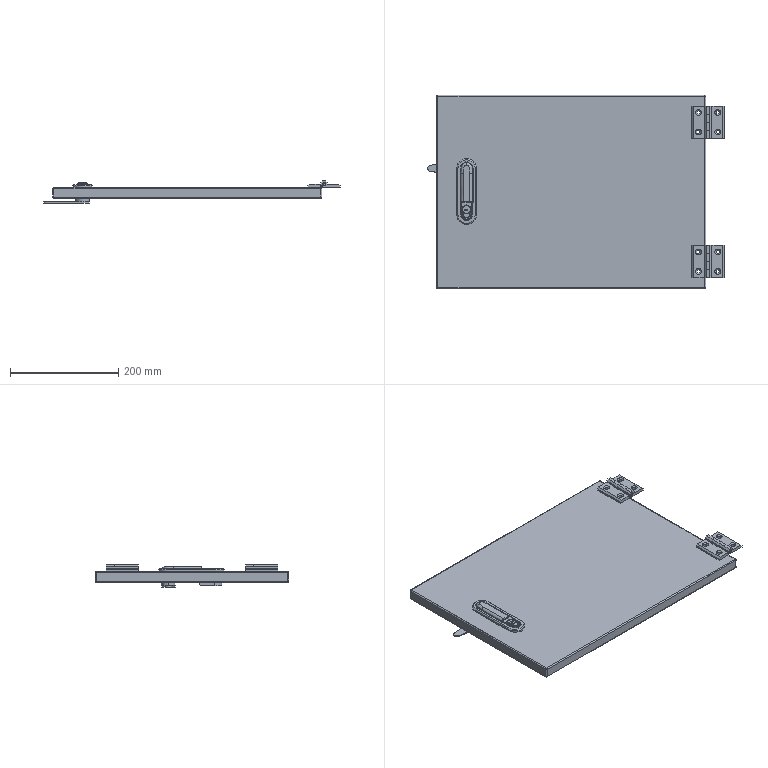Part | SolidWorks | 10 solids | 600 faces | box 549 x 358 x 41 mm | volume 436245 mm3 | plane 270 | cylinder 152 | spline 117 | cone 41 | sphere 16 | torus 4 | commonest cylinder face diameters 1 x22 5.8 x20 2 x17 6.4 x16 4 x15 6.3 x8